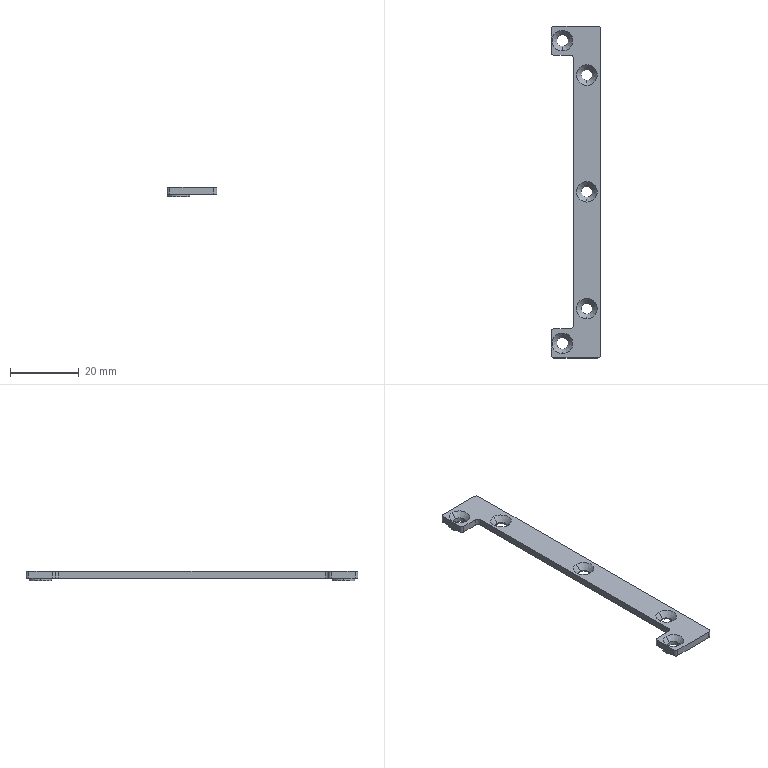NC program | NX | posted with a generic post | part box 14.52 x 96.5 x 2.7 mm
Whole program:
N10 G17 G21 G94 G90
(FLOOR_WALL_COPY , TOOL : D6)
N12 T06 M6
N14 G54
N16 G17 G0 G90 X-59.25 Y7.257 S9500 M3
N18 G43 Z30. H6
N20 Z4.84
N22 G94 G1 Z1.84 F1500.
N24 X-51.25
N26 X51.25
N28 Y4.834
N30 X-51.25
N32 Y2.41
N34 X51.25
N36 Y-0.013
N38 X-51.25
N40 Y-1.069
N42 Y-2.437
N44 X51.25
N46 Y-4.86
N48 X-51.25
N50 X-59.25
N52 Z4.84
N54 G0 Z30.
N56 Y7.257
N58 Z4.38
N60 G1 Z1.38
N62 X-51.25
N64 X51.25
N66 Y4.834
N68 X-51.25
N70 Y2.41
N72 X51.25
N74 Y-0.013
N76 X-51.25
N78 Y-1.069
N80 Y-2.437
N82 X51.25
N84 Y-4.86
N86 X-51.25
N88 X-59.25
N90 Z4.38
N92 G0 Z30.
N94 Y7.257
N96 Z3.92
N98 G1 Z0.92
N100 X-51.25
N102 X51.25
N104 Y4.834
N106 X-51.25
N108 Y2.41
N110 X51.25
N112 Y-0.013
N114 X-51.25
N116 Y-1.069
N118 Y-2.437
N120 X51.25
N122 Y-4.86
N124 X-51.25
N126 X-59.25
N128 Z3.92
N130 G0 Z30.
N132 Y7.257
N134 Z3.46
N136 G1 Z0.46
N138 X-51.25
N140 X51.25
N142 Y4.834
N144 X-51.25
N146 Y2.41
N148 X51.25
N150 Y-0.013
N152 X-51.25
N154 Y-1.069
N156 Y-2.437
N158 X51.25
N160 Y-4.86
N162 X-51.25
N164 X-59.25
N166 Z3.46
N168 G0 Z30.
N170 Y7.257
N172 Z3.
N174 G1 Z0.
N176 X-51.25
N178 X51.25
N180 Y4.834
N182 X-51.25
N184 Y2.41
N186 X51.25
N188 Y-0.013
N190 X-51.25
N192 Y-1.069
N194 Y-2.437
N196 X51.25
N198 Y-4.86
N200 X-51.25
N202 X-59.25
N204 Z3.
N206 G0 Z30.
N208 M5
(FLOOR_WALL_1 , TOOL : D4)
N210 T04 M6
N212 G54
N214 G17 G0 G90 X-1.097 Y10.76 S9500 M3
N216 G43 Z30. H4
N218 Z1.2
N220 G94 G1 Z-0.3 F1000.
N222 X-0.346 Y9.46
N224 G3 X0. Y9.26 R0.4
N226 G1 X47.25 F2500.
N228 G2 X50.25 Y6.26 R3.
N230 G1 Y-6.46
N232 G2 X47.45 Y-9.26 R2.8
N234 G1 X45.084 Y-9.25
N236 G3 X42.916 Y-9.25 R-5.4
N238 G1 X40.55 Y-9.26
N240 G2 X37.75 Y-6.46 R2.8
N242 G1 Y-2.66
N244 X-37.75
N246 Y-6.46
N248 G2 X-40.55 Y-9.26 R2.8
N250 G1 X-42.916 Y-9.25
N252 G3 X-45.084 Y-9.25 R-5.4
N254 G1 X-47.45 Y-9.26
N256 G2 X-50.25 Y-6.46 R2.8
N258 G1 Y6.26
N260 G2 X-47.25 Y9.26 R3.
N262 G1 X0.
N264 Y6.46
N266 X47.25
N268 G2 X47.45 Y6.26 R0.2
N270 G1 Y3.479
N272 G3 X36.899 Y0.14 R8.2
N274 G1 X-36.899
N276 G3 X-47.45 Y3.479 R8.2
N278 G1 Y6.26
N280 G2 X-47.25 Y6.46 R0.2
N282 G1 X0.
N284 Y3.66
N286 X36.067
N288 X38.039 Y4.397
N290 X36.067 Y3.66
N292 G3 X35.433 Y2.94 R11.
N294 G1 X-35.433
N296 G3 X-36.067 Y3.66 R11.
N298 G1 X-38.039 Y4.397
N300 X-36.067 Y3.66
N302 X0.
N304 G3 X0.346 Y3.86 R0.4
N306 G1 Z1.2
N308 G0 Z30.
N310 X-1.097 Y10.76
N312 Z0.9
N314 G1 Z-0.6 F1000.
N316 X-0.346 Y9.46
N318 G3 X0. Y9.26 R0.4
N320 G1 X47.25 F2500.
N322 G2 X50.25 Y6.26 R3.
N324 G1 Y-6.46
N326 G2 X47.45 Y-9.26 R2.8
N328 G1 X45.084 Y-9.25
N330 G3 X42.916 Y-9.25 R-5.4
N332 G1 X40.55 Y-9.26
N334 G2 X37.75 Y-6.46 R2.8
N336 G1 Y-2.66
N338 X-37.75
N340 Y-6.46
N342 G2 X-40.55 Y-9.26 R2.8
N344 G1 X-42.916 Y-9.25
N346 G3 X-45.084 Y-9.25 R-5.4
N348 G1 X-47.45 Y-9.26
N350 G2 X-50.25 Y-6.46 R2.8
N352 G1 Y6.26
N354 G2 X-47.25 Y9.26 R3.
N356 G1 X0.
N358 Y6.46
N360 X47.25
N362 G2 X47.45 Y6.26 R0.2
N364 G1 Y3.479
N366 G3 X36.899 Y0.14 R8.2
N368 G1 X-36.899
N370 G3 X-47.45 Y3.479 R8.2
N372 G1 Y6.26
N374 G2 X-47.25 Y6.46 R0.2
N376 G1 X0.
N378 Y3.66
N380 X36.067
N382 X38.039 Y4.397
N384 X36.067 Y3.66
N386 G3 X35.433 Y2.94 R11.
N388 G1 X-35.433
N390 G3 X-36.067 Y3.66 R11.
N392 G1 X-38.039 Y4.397
N394 X-36.067 Y3.66
N396 X0.
N398 G3 X0.346 Y3.86 R0.4
N400 G1 Z0.9
N402 G0 Z30.
(FLOOR_WALL_1_COPY , TOOL : D4)
N404 X-48.332 Y10.628
N406 Z0.8
N408 G1 Z-0.7 F1000.
N410 X-47.639 Y9.456
N412 G3 X-47.29 Y9.26 R0.4
N414 G1 X-47.273 F1200.
N416 X-47.25
N418 X47.25
N420 G2 X49.32 Y8.432 R3.
N422 G1 X-50.032 Y7.382
N424 G3 X-50.25 Y6.26 R3.
N426 G1 Y5.531
N428 X50.232 Y6.593
N430 G2 X50.25 Y6.26 R3.
N432 G1 Y4.744
N434 X-50.25 Y3.682
N436 Y1.834
N438 X50.25 Y2.895
N440 Y1.047
N442 X46.365 Y1.006
N444 G2 X48.516 Y-0.82 R5.5
N446 G1 X50.25 Y-0.802
N448 Y-2.651
N450 X49.344 Y-2.66
N452 G2 X49.473 Y-4.508 R5.5
N454 G1 X50.25 Y-4.5
N456 Y-6.348
N458 X48.948 Y-6.362
N460 G2 X47.471 Y-8.226 R5.5
N462 G1 X49.641 Y-8.203
N464 G3 X49.985 Y-8. R0.4
N466 G1 X51.553 Y-8.952
N468 Z0.8
N470 G0 Z30.
N472 X-49.373 Y-0.006
N474 Z1.5
N476 G1 X-50.25 Y-0.015 Z1.265 F1000.
N478 X-47.806 Y0.011 Z0.61
N480 X-50.25 Y-0.015 Z-0.045
N482 X-47.806 Y0.011 Z-0.7
N484 X-50.25 Y-0.015 F1200.
N486 Y-1.864
N488 X-49.08 Y-1.851
N490 G3 X-49.494 Y-3.705 R5.5
N492 G1 X-50.25 Y-3.713
N494 Y-5.561
N496 X-49.265 Y-5.551
N498 G3 X-48.3 Y-7.389 R5.5
N500 G1 X-50.085 Y-7.408
N502 G3 X-47.836 Y-9.233 R2.8
N504 G1 X-45.639 Y-9.21
N506 G3 X-46.03 Y-9.298 R0.4
N508 G1 X-48.11 Y-11.214
N510 Z0.8
N512 G0 Z30.
N514 X46.365 Y1.006
N516 Z0.8
N518 G1 Z-0.7 F1000.
N520 G3 X41.531 Y0.954 R5.5
N522 G1 X-40.279 Y0.09 F1200.
N524 G2 X-38.966 Y-1.745 R5.5
N526 G1 X39.419 Y-0.917
N528 G3 X38.629 Y-2.774 R5.5
N530 G1 X37.75 Y-2.783
N532 Y-4.632
N534 X38.54 Y-4.623
N536 G3 X39.104 Y-6.466 R5.5
N538 G1 X37.75 Y-6.48
N540 G3 X38.458 Y-8.322 R2.8
N542 G1 X40.62 Y-8.299
N544 G3 X40.224 Y-8.244 R0.4
N546 G1 X38.941 Y-10.448
N548 Z0.8
N550 G0 Z30.
N552 X-35.75 Y-4.16
N554 Z0.8
N556 G1 Z-0.7 F1000.
N558 X-37.406 Y-3.377
N560 G2 X-37.75 Y-3.581 R0.4
N562 G1 X-38.513 Y-3.589 F1200.
N564 G2 X-38.703 Y-5.439 R5.5
N566 G1 X-37.75 Y-5.429
N568 Y-6.46
N570 G2 X-37.873 Y-7.279 R2.8
N572 G1 X-39.629 Y-7.298
N574 G2 X-42.25 Y-9.174 R5.5
N576 G1 X-39.766 Y-9.148
N578 G3 X-39.422 Y-8.944 R0.4
N580 G1 X-40.254 Y-8.002
N582 G3 X-40.649 Y-8.066 R0.4 F1000.
N584 G2 X-48.106 Y-7.311 R5.3 F1200.
N586 X-40.649 Y-8.066 R-5.3
N588 G3 X-40.791 Y-8.44 R0.4
N590 G1 X-40.531 Y-10.04
N592 Z0.8
N594 G0 Z30.
N596 X45.157 Y-10.864
N598 Z0.8
N600 G1 Z-0.7 F1000.
N602 X44.346 Y-9.46
N604 G3 X44. Y-9.26 R0.4
N606 G2 X38.7 Y-3.96 R5.3 F1200.
N608 X44. Y-9.26 R-5.3
N610 G3 X43.654 Y-9.46 R0.4
N612 G1 X42.843 Y-10.864
N614 Z0.8
N616 G0 Z30.
N618 M5
(PLANAR_MILL_COPY , TOOL : D6A45)
N620 T07 M6
N622 G54
N624 G17 G0 G90 X-44.866 Y0.24 S9500 M3
N626 G43 Z30. H7
N628 Z1.
N630 G94 G1 Z-0.5 F1250.
N632 G3 X-44. Y-0.26 R1.
N634 G2 X-40.3 Y-3.96 R3.7
N636 X-44. Y-0.26 R-3.7
N638 G3 X-43.134 Y0.24 R1.
N640 G1 Z1.
N642 G0 Z30.
N644 Y-3.16
N646 Z1.
N648 G1 Z-0.5
N650 G3 X-44. Y-2.66 R1.
N652 X-45.3 Y-3.96 R1.3
N654 X-44. Y-2.66 R-1.3
N656 X-44.866 Y-3.16 R1.
N658 G1 Z1.
N660 G0 Z30.
N662 X43.134 Y0.24
N664 Z1.
N666 G1 Z-0.5
N668 G3 X44. Y-0.26 R1.
N670 G2 X47.7 Y-3.96 R3.7
N672 X44. Y-0.26 R-3.7
N674 G3 X44.866 Y0.24 R1.
N676 G1 Z1.
N678 G0 Z30.
N680 Y-3.16
N682 Z1.
N684 G1 Z-0.5
N686 G3 X44. Y-2.66 R1.
N688 X42.7 Y-3.96 R1.3
N690 X44. Y-2.66 R-1.3
N692 X43.134 Y-3.16 R1.
N694 G1 Z1.
N696 G0 Z30.
(PLANAR_MILL_COPY_COPY , TOOL : D6A45)
N698 X-33.2 Y3.092
N700 Z-0.2
N702 G1 Y3.269 Z-0.247
N704 X-33.306 Y3.539 Z-0.325
N706 X-33.511 Y3.744 Z-0.403
N708 X-33.781 Y3.85 Z-0.481
N710 X-34.019 Z-0.544
N712 X-34.289 Y3.744 Z-0.622
N714 X-34.494 Y3.539 Z-0.7
N716 X-34.6 Y3.269 Z-0.778
N718 Y3.031 Z-0.841
N720 X-34.494 Y2.761 Z-0.919
N722 X-34.289 Y2.556 Z-0.997
N724 X-34.019 Y2.45 Z-1.074
N726 X-33.781 Z-1.138
N728 X-33.511 Y2.556 Z-1.216
N730 X-33.306 Y2.761 Z-1.294
N732 X-33.2 Y3.031 Z-1.371
N734 Y3.269 Z-1.435
N736 X-33.306 Y3.539 Z-1.513
N738 X-33.511 Y3.744 Z-1.59
N740 X-33.781 Y3.85 Z-1.668
N742 X-33.9 Z-1.7
N744 G3 X-34.6 Y3.15 R0.7
N746 X-33.9 Y3.85 R-0.7
N748 X-34.333 Y3.6 R0.5
N750 G1 Z-0.2
N752 G0 Z30.
N754 X0.75 Y3.092
N756 Z-0.2
N758 G1 Y3.269 Z-0.247
N760 X0.644 Y3.539 Z-0.325
N762 X0.439 Y3.744 Z-0.403
N764 X0.169 Y3.85 Z-0.481
N766 X-0.069 Z-0.544
N768 X-0.339 Y3.744 Z-0.622
N770 X-0.544 Y3.539 Z-0.7
N772 X-0.65 Y3.269 Z-0.778
N774 Y3.031 Z-0.841
N776 X-0.544 Y2.761 Z-0.919
N778 X-0.339 Y2.556 Z-0.997
N780 X-0.069 Y2.45 Z-1.074
N782 X0.169 Z-1.138
N784 X0.439 Y2.556 Z-1.216
N786 X0.644 Y2.761 Z-1.294
N788 X0.75 Y3.031 Z-1.371
N790 Y3.269 Z-1.435
N792 X0.644 Y3.539 Z-1.513
N794 X0.439 Y3.744 Z-1.59
N796 X0.169 Y3.85 Z-1.668
N798 X0.05 Z-1.7
N800 G3 X-0.65 Y3.15 R0.7
N802 X0.05 Y3.85 R-0.7
N804 X-0.383 Y3.6 R0.5
N806 G1 Z-0.2
N808 G0 Z30.
N810 X37.405 Y-2.777
N812 Z-0.2
N814 G1 Z-1.7
N816 X38.078 Y-2.665
N818 G3 X38.85 Y-2.029 R1.
N820 G1 Y-1.66
N822 X38.845 Y-1.605
N824 X38.805 Y-1.565
N826 X38.75 Y-1.56
N828 X-38.75
N830 X-38.805 Y-1.565
N832 X-38.845 Y-1.605
N834 X-38.85 Y-1.66
N836 Y-2.029
N838 G3 X-38.078 Y-2.665 R1.
N840 G1 Y-5.255
N842 G3 X-38.85 Y-5.891 R1.
N844 G1 Y-6.46
N846 G2 X-40.445 Y-8.157 R1.7
N848 G3 X-40.783 Y-9.098 R1.
N850 G1 X-40.661 Y-9.769
N852 Z-0.2
N854 G0 Z30.
N856 X-47.339
N858 Z-0.2
N860 G1 Z-1.7
N862 X-47.217 Y-9.098
N864 G3 X-47.555 Y-8.157 R1.
N866 G2 X-49.15 Y-6.46 R1.7
N868 G1 Y-5.891
N870 G3 X-49.922 Y-5.255 R1.
N872 G1 Y-2.665
N874 G3 X-49.15 Y-2.029 R1.
N876 G1 Y6.26
N878 G2 X-47.25 Y8.16 R1.9
N880 G1 X47.25
N882 G2 X49.15 Y6.26 R1.9
N884 G1 Y-2.029
N886 G3 X49.922 Y-2.665 R1.
N888 G1 Y-5.255
N890 G3 X49.15 Y-5.891 R1.
N892 G1 Y-6.46
N894 G2 X47.555 Y-8.157 R1.7
N896 G3 X47.217 Y-9.098 R1.
N898 G1 X47.339 Y-9.769
N900 Z-0.2
N902 G0 Z30.
N904 X40.661
N906 Z-0.2
N908 G1 Z-1.7
N910 X40.783 Y-9.098
N912 G3 X40.445 Y-8.157 R1.
N914 G2 X38.85 Y-6.46 R1.7
N916 G1 Y-5.891
N918 G3 X38.078 Y-5.255 R1.
N920 G1 X37.405 Y-5.143
N922 Z-0.2
N924 G0 Z30.
N926 X34.7 Y3.092
N928 Z-0.2
N930 G1 Y3.269 Z-0.247
N932 X34.594 Y3.539 Z-0.325
N934 X34.389 Y3.744 Z-0.403
N936 X34.119 Y3.85 Z-0.481
N938 X33.881 Z-0.544
N940 X33.611 Y3.744 Z-0.622
N942 X33.406 Y3.539 Z-0.7
N944 X33.3 Y3.269 Z-0.778
N946 Y3.031 Z-0.841
N948 X33.406 Y2.761 Z-0.919
N950 X33.611 Y2.556 Z-0.997
N952 X33.881 Y2.45 Z-1.074
N954 X34.119 Z-1.138
N956 X34.389 Y2.556 Z-1.216
N958 X34.594 Y2.761 Z-1.294
N960 X34.7 Y3.031 Z-1.371
N962 Y3.269 Z-1.435
N964 X34.594 Y3.539 Z-1.513
N966 X34.389 Y3.744 Z-1.59
N968 X34.119 Y3.85 Z-1.668
N970 X34. Z-1.7
N972 G3 X33.3 Y3.15 R0.7
N974 X34. Y3.85 R-0.7
N976 X33.567 Y3.6 R0.5
N978 G1 Z-0.2
N980 G0 Z30.
N982 M5
N984 M2